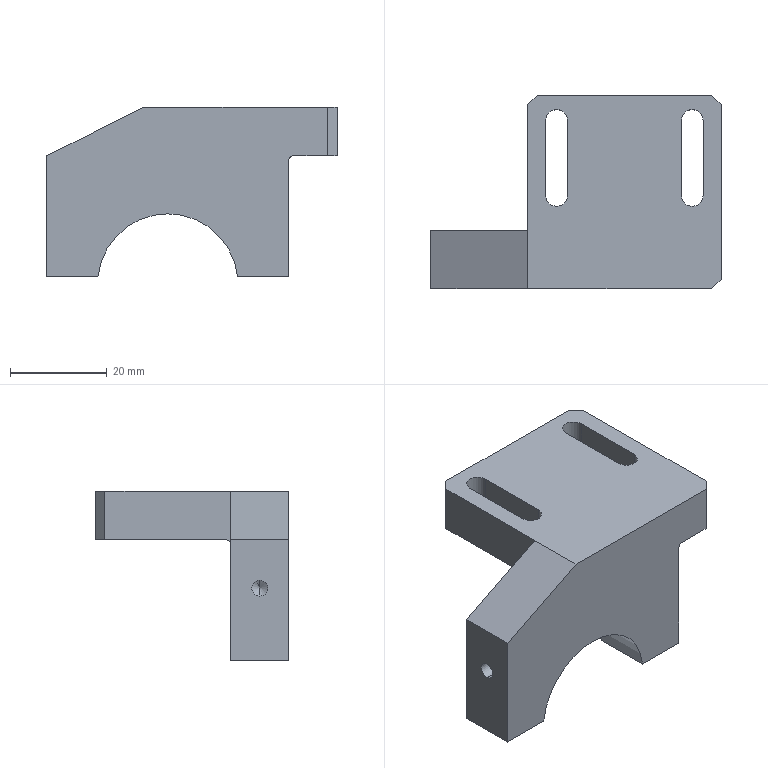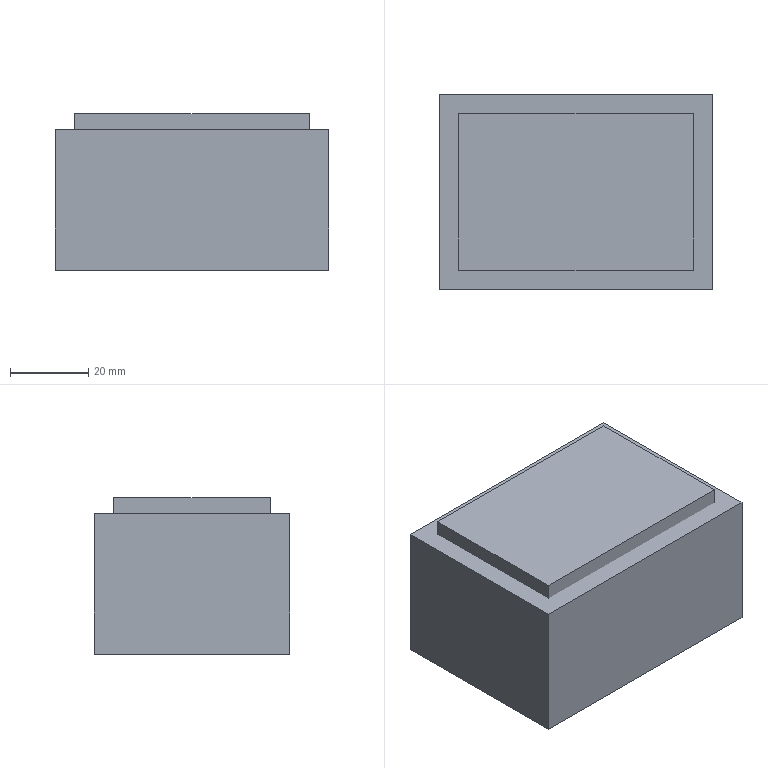CAM job | NX | 3-axis milling, drilling | part box 60 x 40 x 35 mm | stock box 70 x 50 x 40 mm
Tools:
number,name,description,diameter,corner_radius,flute_length,length,flutes
19,D80,Milling Tool-5 Parameters,80.0,0.0,50.0,75.0,2
1,D6A45,Milling Tool-5 Parameters,6.0,0.0,50.0,75.0,2
3,3.3ZT,Drilling Tool,3.3,0.0,35.0,50.0,2
15,D10,Milling Tool-5 Parameters,10.0,0.0,50.0,75.0,2
14,D10JING,Milling Tool-5 Parameters,10.0,0.0,50.0,75.0,2
12,D6,Milling Tool-5 Parameters,6.0,0.0,50.0,75.0,2
16,D6R0.5,Milling Tool-5 Parameters,6.0,0.5,50.0,75.0,2
18,R2,Milling Tool-5 Parameters,4.0,2.0,50.0,75.0,2
11,D4,Milling Tool-5 Parameters,4.0,0.0,50.0,75.0,2
Operations:
program,operation,operation_type,tool,method,geometry_group,spindle_rpm,surface_speed,feed_per_tooth,feed_cut,feed_plunge,cut_length_mm,path_length_mm,cut_time_min,machine_time_min
1,FLOOR_WALL,VolumeBased25DMillingOperation,D80,METHOD,A,6500.0,1633.0,0.1154,1500.0,100.0,162.0,216.0,0.108,0.1134
1,DRILLING,Operation,D6A45,METHOD,A,5000.0,94.0,0.035,350.0,0.0,8.0,119.112,0.0229,0.034
1,DRILLING_COPY_1,Operation,3.3ZT,METHOD,A,2000.0,20.0,0.05,200.0,0.0,30.983,165.078,0.1549,0.1683
1,ADAPTIVE_MILLING,CavityMilling,D10,METHOD,A,9500.0,298.0,0.1842,3500.0,1000.0,10738.879,10983.932,3.072,3.097
1,FLOOR_WALL_1,VolumeBased25DMillingOperation,D10,METHOD,A,9500.0,298.0,0.1842,3500.0,1000.0,3103.273,3370.22,0.8993,0.926
1,PLANAR_MILL,PlanarMilling,D10,METHOD,A,9500.0,298.0,0.1579,3000.0,100.0,1405.669,4386.811,0.4686,0.7667
1,FIXED_CONTOUR,SurfaceContour,D10,METHOD,A,9500.0,298.0,0.1316,2500.0,100.0,3299.726,3337.768,1.32,1.324
1,ZLEVEL_PROFILE_COPY_1,ZLevelMilling,D10JING,METHOD,A,9500.0,298.0,0.0632,1200.0,1000.0,1017.455,1214.847,0.9335,0.9533
1,ZLEVEL_PROFILE_COPY_1_COPY,ZLevelMilling,D10JING,METHOD,A,9500.0,298.0,0.0632,1200.0,1000.0,446.989,563.989,0.4091,0.4208
1,FLOOR_WALL_2,VolumeBased25DMillingOperation,D10JING,METHOD,A,9500.0,298.0,0.0789,1500.0,100.0,464.107,686.186,0.3094,0.3316
1,ZLEVEL_PROFILE_COPY_1_COPY_COPY,ZLevelMilling,D6,METHOD,A,9500.0,179.0,0.0632,1200.0,1000.0,283.831,514.025,0.246,0.269
1,ZLEVEL_PROFILE,ZLevelMilling,D6,METHOD,A,6000.0,113.0,0.1,1200.0,1000.0,1040.505,1291.742,0.8791,0.9042
1,ZLEVEL_PROFILE_1,ZLevelMilling,D6R0.5,METHOD,A,7500.0,141.0,0.1333,2000.0,100.0,1117.312,1224.412,0.5587,0.5694
1,FIXED_CONTOUR_COPY,SurfaceContour,R2,METHOD,A,9500.0,119.0,0.1579,3000.0,100.0,4420.44,4476.44,1.474,1.479
1,PLANAR_MILL_COPY_COPY_COPY,PlanarMilling,D6A45,METHOD,A,9500.0,179.0,0.0658,1250.0,100.0,129.329,426.104,0.1035,0.1331
1,PLANAR_MILL_COPY_COPY_COPY_COPY,PlanarMilling,D6A45,METHOD,A,9500.0,179.0,0.0658,1250.0,100.0,227.701,620.994,0.1822,0.2215
2,FLOOR_WALL_COPY,VolumeBased25DMillingOperation,D80,METHOD,B,6500.0,1633.0,0.1154,1500.0,100.0,760.0,1594.001,0.5067,0.5901
2,ZLEVEL_PROFILE_1_COPY_COPY,ZLevelMilling,D10,METHOD,B,7500.0,141.0,0.1333,2000.0,100.0,1108.67,1177.393,0.5543,0.5612
2,ZLEVEL_PROFILE_1_COPY,ZLevelMilling,D6R0.5,METHOD,B,7500.0,141.0,0.1333,2000.0,100.0,4255.003,4323.547,2.127,2.134
2,ZLEVEL_PROFILE_COPY,ZLevelMilling,D4,METHOD,B,9000.0,113.0,0.1111,2000.0,1000.0,1051.285,1204.712,0.5619,0.5773
2,PLANAR_MILL_COPY_COPY_COPY_COPY_COPY,PlanarMilling,D6A45,METHOD,B,9500.0,179.0,0.0658,1250.0,100.0,244.813,481.096,0.1959,0.2195